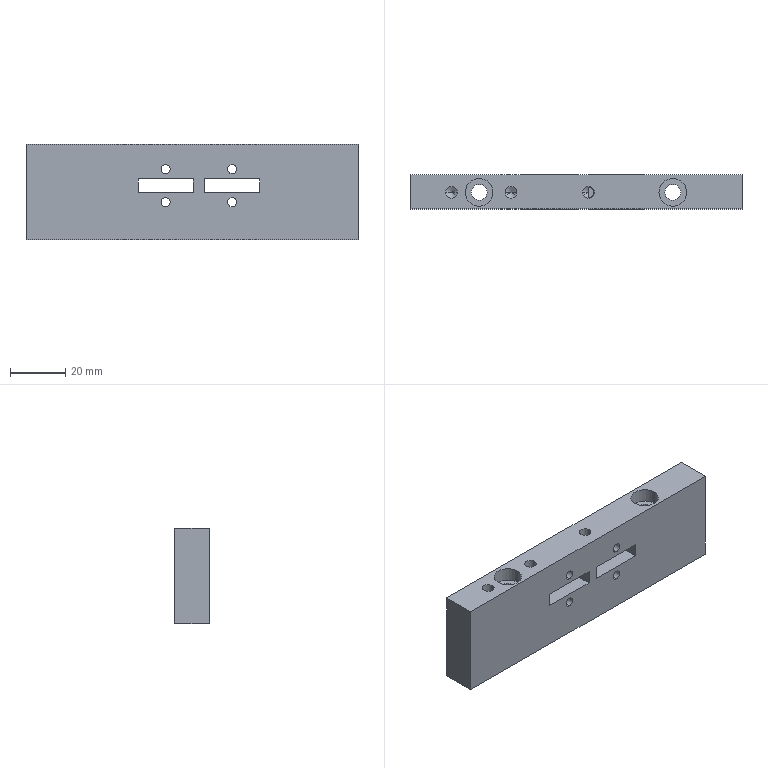Part | STEP file | magnetizing side block 2 | 1 solid | 44 faces | box 120 x 12.3 x 34.5 mm | volume 45166 mm3 | cylinder 22 | plane 16 | cone 6 | commonest cylinder face diameters 3.3 x8 4.2 x6 5.8 x4 10 x4